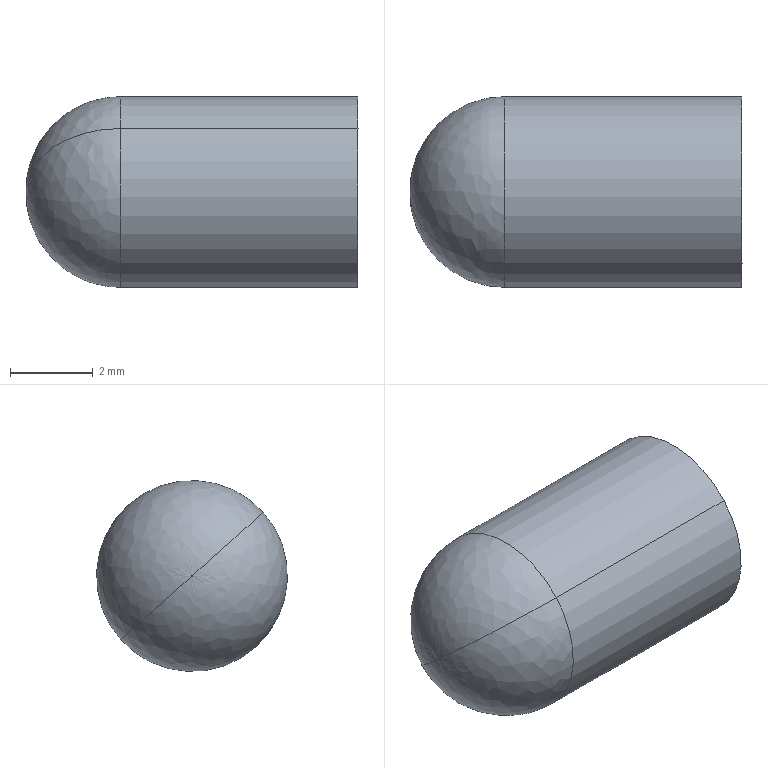Part | NX | features solid 2 | 1 solid | 11 faces | box 8 x 4.6 x 4.6 mm | volume 85.487 mm3 | cylinder 4 | plane 3 | spline 2 | cone 2 | commonest cylinder face diameters 2.6 x2 4.6 x2
STEP:
#1=CARTESIAN_POINT('',(270.755,52.052,28.635));
#2=VERTEX_POINT('',#1);
#3=CARTESIAN_POINT('',(276.475,52.052,28.635));
#4=VERTEX_POINT('',#3);
#5=CARTESIAN_POINT('',(276.475,52.052,28.635));
#6=DIRECTION('',(-1.,0.,0.));
#7=VECTOR('',#6,1000.);
#8=LINE('',#5,#7);
#9=EDGE_CURVE('',#2,#4,#8,.F.);
#10=ORIENTED_EDGE('',*,*,#9,.T.);
#11=CARTESIAN_POINT('',(276.475,55.486,25.575));
#12=VERTEX_POINT('',#11);
#13=CARTESIAN_POINT('',(276.475,53.769,27.105));
#14=DIRECTION('',(1.,0.,0.));
#15=DIRECTION('',(0.,0.7465,-0.6654));
#16=AXIS2_PLACEMENT_3D('',#13,#14,#15);
#17=CIRCLE('',#16,2.3);
#18=EDGE_CURVE('',#12,#4,#17,.T.);
#19=ORIENTED_EDGE('',*,*,#18,.F.);
#20=CARTESIAN_POINT('',(270.755,55.486,25.575));
#21=VERTEX_POINT('',#20);
#22=CARTESIAN_POINT('',(276.475,55.486,25.575));
#23=DIRECTION('',(-1.,0.,0.));
#24=VECTOR('',#23,1000.);
#25=LINE('',#22,#24);
#26=EDGE_CURVE('',#12,#21,#25,.T.);
#27=ORIENTED_EDGE('',*,*,#26,.T.);
#28=CARTESIAN_POINT('',(270.755,53.769,27.105));
#29=DIRECTION('',(-1.,0.,0.));
#30=DIRECTION('',(0.,-0.7465,0.6654));
#31=AXIS2_PLACEMENT_3D('',#28,#29,#30);
#32=CIRCLE('',#31,2.3);
#33=EDGE_CURVE('',#2,#21,#32,.T.);
#34=ORIENTED_EDGE('',*,*,#33,.F.);
#35=EDGE_LOOP('',(#10,#19,#27,#34));
#36=FACE_BOUND('',#35,.T.);
#37=CARTESIAN_POINT('',(276.475,53.769,27.105));
#38=DIRECTION('',(-1.,0.,0.));
#39=DIRECTION('',(0.,0.7465,-0.6654));
#40=AXIS2_PLACEMENT_3D('',#37,#38,#39);
#41=CYLINDRICAL_SURFACE('',#40,2.3);
#42=ADVANCED_FACE('',(#36),#41,.T.);
#43=CARTESIAN_POINT('',(268.475,53.755,27.118));
#44=VERTEX_POINT('',#43);
#45=CARTESIAN_POINT('',(270.755,53.755,27.118));
#46=DIRECTION('',(0.,0.6654,0.7465));
#47=DIRECTION('',(-1.,0.,0.));
#48=AXIS2_PLACEMENT_3D('',#45,#46,#47);
#49=CIRCLE('',#48,2.28);
#50=EDGE_CURVE('',#2,#44,#49,.F.);
#51=ORIENTED_EDGE('',*,*,#50,.F.);
#52=ORIENTED_EDGE('',*,*,#33,.T.);
#53=CARTESIAN_POINT('',(268.475,53.784,27.092));
#54=VERTEX_POINT('',#53);
#55=CARTESIAN_POINT('',(270.755,53.784,27.092));
#56=DIRECTION('',(0.,-0.6654,-0.7465));
#57=DIRECTION('',(-1.,0.,0.));
#58=AXIS2_PLACEMENT_3D('',#55,#56,#57);
#59=CIRCLE('',#58,2.28);
#60=EDGE_CURVE('',#54,#21,#59,.T.);
#61=ORIENTED_EDGE('',*,*,#60,.F.);
#62=CARTESIAN_POINT('',(268.475,53.769,27.105));
#63=DIRECTION('',(-1.,0.,0.));
#64=DIRECTION('',(0.,-0.7465,0.6654));
#65=AXIS2_PLACEMENT_3D('',#62,#63,#64);
#66=CIRCLE('',#65,0.01975);
#67=EDGE_CURVE('',#44,#54,#66,.T.);
#68=ORIENTED_EDGE('',*,*,#67,.F.);
#69=EDGE_LOOP('',(#51,#52,#61,#68));
#70=FACE_BOUND('',#69,.T.);
#71=CARTESIAN_POINT('',(268.475,53.77,27.095));
#72=CARTESIAN_POINT('',(268.469,53.911,25.728));
#73=CARTESIAN_POINT('',(269.454,54.009,24.775));
#74=CARTESIAN_POINT('',(270.827,54.005,24.818));
#75=CARTESIAN_POINT('',(268.475,53.78,27.096));
#76=CARTESIAN_POINT('',(268.469,55.305,25.872));
#77=CARTESIAN_POINT('',(269.454,56.369,25.018));
#78=CARTESIAN_POINT('',(270.827,56.321,25.057));
#79=CARTESIAN_POINT('',(268.475,53.783,27.106));
#80=CARTESIAN_POINT('',(268.469,55.736,27.205));
#81=CARTESIAN_POINT('',(269.454,57.098,27.275));
#82=CARTESIAN_POINT('',(270.827,57.037,27.272));
#83=CARTESIAN_POINT('',(268.475,53.776,27.112));
#84=CARTESIAN_POINT('',(268.469,54.69,28.138));
#85=CARTESIAN_POINT('',(269.454,55.328,28.853));
#86=CARTESIAN_POINT('',(270.827,55.299,28.821));
#87=CARTESIAN_POINT('',(268.475,53.768,27.119));
#88=CARTESIAN_POINT('',(268.469,53.644,29.071));
#89=CARTESIAN_POINT('',(269.454,53.557,30.432));
#90=CARTESIAN_POINT('',(270.827,53.561,30.37));
#91=CARTESIAN_POINT('',(268.475,53.759,27.115));
#92=CARTESIAN_POINT('',(268.469,52.369,28.489));
#93=CARTESIAN_POINT('',(269.454,51.398,29.448));
#94=CARTESIAN_POINT('',(270.827,51.442,29.405));
#95=CARTESIAN_POINT('',(268.475,53.759,27.105));
#96=CARTESIAN_POINT('',(268.469,52.386,27.088));
#97=CARTESIAN_POINT('',(269.454,51.427,27.076));
#98=CARTESIAN_POINT('',(270.827,51.471,27.077));
#99=(BOUNDED_SURFACE()B_SPLINE_SURFACE(3,3,((#71,#72,#73,#74),(#75,#76,#77,#78),(#79,#80,#81,#82),(#83,#84,#85,#86),(#87,#88,#89,#90),(#91,#92,#93,#94),(#95,#96,#97,#98)),.UNSPECIFIED.,.F.,.F.,.F.)B_SPLINE_SURFACE_WITH_KNOTS((4,3,4),(4,4),(0.,0.5,1.),(0.,1.),.PIECEWISE_BEZIER_KNOTS.)GEOMETRIC_REPRESENTATION_ITEM()RATIONAL_B_SPLINE_SURFACE(((1.682,1.339,1.339,1.682),(1.013,0.8067,0.8067,1.013),(1.013,0.8067,0.8067,1.013),(1.682,1.339,1.339,1.682),(1.013,0.8067,0.8067,1.013),(1.013,0.8067,0.8067,1.013),(1.682,1.339,1.339,1.682)))REPRESENTATION_ITEM('')SURFACE());
#100=ADVANCED_FACE('',(#70),#99,.T.);
#101=CARTESIAN_POINT('',(268.475,53.769,27.105));
#102=DIRECTION('',(-1.,0.,0.));
#103=DIRECTION('',(0.,0.7465,-0.6654));
#104=AXIS2_PLACEMENT_3D('',#101,#102,#103);
#105=CIRCLE('',#104,0.01975);
#106=EDGE_CURVE('',#54,#44,#105,.T.);
#107=ORIENTED_EDGE('',*,*,#106,.T.);
#108=ORIENTED_EDGE('',*,*,#67,.T.);
#109=EDGE_LOOP('',(#107,#108));
#110=FACE_BOUND('',#109,.T.);
#111=CARTESIAN_POINT('',(268.475,53.782,27.12));
#112=DIRECTION('',(1.,0.,0.));
#113=DIRECTION('',(0.,-0.7465,0.6654));
#114=AXIS2_PLACEMENT_3D('',#111,#112,#113);
#115=PLANE('',#114);
#116=ADVANCED_FACE('',(#110),#115,.F.);
#117=ORIENTED_EDGE('',*,*,#60,.T.);
#118=CARTESIAN_POINT('',(270.755,53.769,27.105));
#119=DIRECTION('',(-1.,0.,0.));
#120=DIRECTION('',(0.,0.7465,-0.6654));
#121=AXIS2_PLACEMENT_3D('',#118,#119,#120);
#122=CIRCLE('',#121,2.3);
#123=EDGE_CURVE('',#21,#2,#122,.T.);
#124=ORIENTED_EDGE('',*,*,#123,.T.);
#125=ORIENTED_EDGE('',*,*,#50,.T.);
#126=ORIENTED_EDGE('',*,*,#106,.F.);
#127=EDGE_LOOP('',(#117,#124,#125,#126));
#128=FACE_BOUND('',#127,.T.);
#129=CARTESIAN_POINT('',(268.475,53.768,27.115));
#130=CARTESIAN_POINT('',(268.469,53.628,28.482));
#131=CARTESIAN_POINT('',(269.454,53.53,29.435));
#132=CARTESIAN_POINT('',(270.827,53.534,29.392));
#133=CARTESIAN_POINT('',(268.475,53.758,27.114));
#134=CARTESIAN_POINT('',(268.469,52.234,28.338));
#135=CARTESIAN_POINT('',(269.454,51.17,29.192));
#136=CARTESIAN_POINT('',(270.827,51.218,29.153));
#137=CARTESIAN_POINT('',(268.475,53.755,27.104));
#138=CARTESIAN_POINT('',(268.469,51.802,27.005));
#139=CARTESIAN_POINT('',(269.454,50.44,26.935));
#140=CARTESIAN_POINT('',(270.827,50.502,26.938));
#141=CARTESIAN_POINT('',(268.475,53.763,27.098));
#142=CARTESIAN_POINT('',(268.469,52.849,26.072));
#143=CARTESIAN_POINT('',(269.454,52.211,25.357));
#144=CARTESIAN_POINT('',(270.827,52.24,25.389));
#145=CARTESIAN_POINT('',(268.475,53.77,27.091));
#146=CARTESIAN_POINT('',(268.469,53.895,25.139));
#147=CARTESIAN_POINT('',(269.454,53.982,23.778));
#148=CARTESIAN_POINT('',(270.827,53.978,23.84));
#149=CARTESIAN_POINT('',(268.475,53.779,27.095));
#150=CARTESIAN_POINT('',(268.469,55.17,25.721));
#151=CARTESIAN_POINT('',(269.454,56.14,24.762));
#152=CARTESIAN_POINT('',(270.827,56.096,24.805));
#153=CARTESIAN_POINT('',(268.475,53.779,27.105));
#154=CARTESIAN_POINT('',(268.469,55.153,27.122));
#155=CARTESIAN_POINT('',(269.454,56.111,27.134));
#156=CARTESIAN_POINT('',(270.827,56.068,27.133));
#157=(BOUNDED_SURFACE()B_SPLINE_SURFACE(3,3,((#129,#130,#131,#132),(#133,#134,#135,#136),(#137,#138,#139,#140),(#141,#142,#143,#144),(#145,#146,#147,#148),(#149,#150,#151,#152),(#153,#154,#155,#156)),.UNSPECIFIED.,.F.,.F.,.F.)B_SPLINE_SURFACE_WITH_KNOTS((4,3,4),(4,4),(0.,0.5,1.),(0.,1.),.PIECEWISE_BEZIER_KNOTS.)GEOMETRIC_REPRESENTATION_ITEM()RATIONAL_B_SPLINE_SURFACE(((1.682,1.339,1.339,1.682),(1.013,0.8067,0.8067,1.013),(1.013,0.8067,0.8067,1.013),(1.682,1.339,1.339,1.682),(1.013,0.8067,0.8067,1.013),(1.013,0.8067,0.8067,1.013),(1.682,1.339,1.339,1.682)))REPRESENTATION_ITEM('')SURFACE());
#158=ADVANCED_FACE('',(#128),#157,.T.);
#159=ORIENTED_EDGE('',*,*,#26,.F.);
#160=CARTESIAN_POINT('',(276.475,53.769,27.105));
#161=DIRECTION('',(1.,0.,0.));
#162=DIRECTION('',(0.,-0.7465,0.6654));
#163=AXIS2_PLACEMENT_3D('',#160,#161,#162);
#164=CIRCLE('',#163,2.3);
#165=EDGE_CURVE('',#4,#12,#164,.T.);
#166=ORIENTED_EDGE('',*,*,#165,.F.);
#167=ORIENTED_EDGE('',*,*,#9,.F.);
#168=ORIENTED_EDGE('',*,*,#123,.F.);
#169=EDGE_LOOP('',(#159,#166,#167,#168));
#170=FACE_BOUND('',#169,.T.);
#171=CARTESIAN_POINT('',(276.475,53.769,27.105));
#172=DIRECTION('',(-1.,0.,0.));
#173=DIRECTION('',(0.,0.7465,-0.6654));
#174=AXIS2_PLACEMENT_3D('',#171,#172,#173);
#175=CYLINDRICAL_SURFACE('',#174,2.3);
#176=ADVANCED_FACE('',(#170),#175,.T.);
#177=ORIENTED_EDGE('',*,*,#18,.T.);
#178=ORIENTED_EDGE('',*,*,#165,.T.);
#179=EDGE_LOOP('',(#177,#178));
#180=FACE_BOUND('',#179,.T.);
#181=CARTESIAN_POINT('',(276.475,54.964,26.04));
#182=VERTEX_POINT('',#181);
#183=CARTESIAN_POINT('',(276.475,52.575,28.17));
#184=VERTEX_POINT('',#183);
#185=CARTESIAN_POINT('',(276.475,53.769,27.105));
#186=DIRECTION('',(-1.,0.,0.));
#187=DIRECTION('',(0.,0.7465,-0.6654));
#188=AXIS2_PLACEMENT_3D('',#185,#186,#187);
#189=CIRCLE('',#188,1.6);
#190=EDGE_CURVE('',#182,#184,#189,.T.);
#191=ORIENTED_EDGE('',*,*,#190,.T.);
#192=CARTESIAN_POINT('',(276.475,53.769,27.105));
#193=DIRECTION('',(-1.,0.,0.));
#194=DIRECTION('',(0.,-0.7465,0.6654));
#195=AXIS2_PLACEMENT_3D('',#192,#193,#194);
#196=CIRCLE('',#195,1.6);
#197=EDGE_CURVE('',#184,#182,#196,.T.);
#198=ORIENTED_EDGE('',*,*,#197,.T.);
#199=EDGE_LOOP('',(#191,#198));
#200=FACE_BOUND('',#199,.T.);
#201=CARTESIAN_POINT('',(276.475,54.634,28.075));
#202=DIRECTION('',(-1.,0.,0.));
#203=DIRECTION('',(0.,0.7465,-0.6654));
#204=AXIS2_PLACEMENT_3D('',#201,#202,#203);
#205=PLANE('',#204);
#206=ADVANCED_FACE('',(#180,#200),#205,.F.);
#207=CARTESIAN_POINT('',(276.175,54.74,26.24));
#208=VERTEX_POINT('',#207);
#209=CARTESIAN_POINT('',(276.175,54.74,26.24));
#210=DIRECTION('',(0.7071,0.5279,-0.4705));
#211=VECTOR('',#210,1000.);
#212=LINE('',#209,#211);
#213=EDGE_CURVE('',#182,#208,#212,.F.);
#214=ORIENTED_EDGE('',*,*,#213,.F.);
#215=ORIENTED_EDGE('',*,*,#197,.F.);
#216=CARTESIAN_POINT('',(276.175,52.799,27.97));
#217=VERTEX_POINT('',#216);
#218=CARTESIAN_POINT('',(276.175,52.799,27.97));
#219=DIRECTION('',(0.7071,-0.5279,0.4705));
#220=VECTOR('',#219,1000.);
#221=LINE('',#218,#220);
#222=EDGE_CURVE('',#217,#184,#221,.T.);
#223=ORIENTED_EDGE('',*,*,#222,.F.);
#224=CARTESIAN_POINT('',(276.175,53.769,27.105));
#225=DIRECTION('',(-1.,0.,0.));
#226=DIRECTION('',(0.,-0.7465,0.6654));
#227=AXIS2_PLACEMENT_3D('',#224,#225,#226);
#228=CIRCLE('',#227,1.3);
#229=EDGE_CURVE('',#217,#208,#228,.T.);
#230=ORIENTED_EDGE('',*,*,#229,.T.);
#231=EDGE_LOOP('',(#214,#215,#223,#230));
#232=FACE_BOUND('',#231,.T.);
#233=CARTESIAN_POINT('',(276.325,53.769,27.105));
#234=DIRECTION('',(1.,0.,0.));
#235=DIRECTION('',(0.,-0.7465,0.6654));
#236=AXIS2_PLACEMENT_3D('',#233,#234,#235);
#237=CONICAL_SURFACE('',#236,1.45,0.7854);
#238=ADVANCED_FACE('',(#232),#237,.F.);
#239=CARTESIAN_POINT('',(269.975,52.799,27.97));
#240=VERTEX_POINT('',#239);
#241=CARTESIAN_POINT('',(276.175,52.799,27.97));
#242=DIRECTION('',(-1.,0.,0.));
#243=VECTOR('',#242,1000.);
#244=LINE('',#241,#243);
#245=EDGE_CURVE('',#217,#240,#244,.T.);
#246=ORIENTED_EDGE('',*,*,#245,.T.);
#247=CARTESIAN_POINT('',(269.975,54.74,26.24));
#248=VERTEX_POINT('',#247);
#249=CARTESIAN_POINT('',(269.975,53.769,27.105));
#250=DIRECTION('',(1.,0.,0.));
#251=DIRECTION('',(0.,0.7465,-0.6654));
#252=AXIS2_PLACEMENT_3D('',#249,#250,#251);
#253=CIRCLE('',#252,1.3);
#254=EDGE_CURVE('',#248,#240,#253,.T.);
#255=ORIENTED_EDGE('',*,*,#254,.F.);
#256=CARTESIAN_POINT('',(276.175,54.74,26.24));
#257=DIRECTION('',(-1.,0.,0.));
#258=VECTOR('',#257,1000.);
#259=LINE('',#256,#258);
#260=EDGE_CURVE('',#248,#208,#259,.F.);
#261=ORIENTED_EDGE('',*,*,#260,.T.);
#262=ORIENTED_EDGE('',*,*,#229,.F.);
#263=EDGE_LOOP('',(#246,#255,#261,#262));
#264=FACE_BOUND('',#263,.T.);
#265=CARTESIAN_POINT('',(276.475,53.769,27.105));
#266=DIRECTION('',(-1.,0.,0.));
#267=DIRECTION('',(0.,0.7465,-0.6654));
#268=AXIS2_PLACEMENT_3D('',#265,#266,#267);
#269=CYLINDRICAL_SURFACE('',#268,1.3);
#270=ADVANCED_FACE('',(#264),#269,.F.);
#271=ORIENTED_EDGE('',*,*,#260,.F.);
#272=CARTESIAN_POINT('',(269.975,53.769,27.105));
#273=DIRECTION('',(1.,0.,0.));
#274=DIRECTION('',(0.,-0.7465,0.6654));
#275=AXIS2_PLACEMENT_3D('',#272,#273,#274);
#276=CIRCLE('',#275,1.3);
#277=EDGE_CURVE('',#240,#248,#276,.T.);
#278=ORIENTED_EDGE('',*,*,#277,.F.);
#279=ORIENTED_EDGE('',*,*,#245,.F.);
#280=CARTESIAN_POINT('',(276.175,53.769,27.105));
#281=DIRECTION('',(-1.,0.,0.));
#282=DIRECTION('',(0.,0.7465,-0.6654));
#283=AXIS2_PLACEMENT_3D('',#280,#281,#282);
#284=CIRCLE('',#283,1.3);
#285=EDGE_CURVE('',#208,#217,#284,.T.);
#286=ORIENTED_EDGE('',*,*,#285,.F.);
#287=EDGE_LOOP('',(#271,#278,#279,#286));
#288=FACE_BOUND('',#287,.T.);
#289=CARTESIAN_POINT('',(276.475,53.769,27.105));
#290=DIRECTION('',(-1.,0.,0.));
#291=DIRECTION('',(0.,0.7465,-0.6654));
#292=AXIS2_PLACEMENT_3D('',#289,#290,#291);
#293=CYLINDRICAL_SURFACE('',#292,1.3);
#294=ADVANCED_FACE('',(#288),#293,.F.);
#295=ORIENTED_EDGE('',*,*,#222,.T.);
#296=ORIENTED_EDGE('',*,*,#190,.F.);
#297=ORIENTED_EDGE('',*,*,#213,.T.);
#298=ORIENTED_EDGE('',*,*,#285,.T.);
#299=EDGE_LOOP('',(#295,#296,#297,#298));
#300=FACE_BOUND('',#299,.T.);
#301=CARTESIAN_POINT('',(276.325,53.769,27.105));
#302=DIRECTION('',(1.,0.,0.));
#303=DIRECTION('',(0.,-0.7465,0.6654));
#304=AXIS2_PLACEMENT_3D('',#301,#302,#303);
#305=CONICAL_SURFACE('',#304,1.45,0.7854);
#306=ADVANCED_FACE('',(#300),#305,.F.);
#307=ORIENTED_EDGE('',*,*,#254,.T.);
#308=ORIENTED_EDGE('',*,*,#277,.T.);
#309=EDGE_LOOP('',(#307,#308));
#310=FACE_BOUND('',#309,.T.);
#311=CARTESIAN_POINT('',(269.975,53.769,27.105));
#312=DIRECTION('',(-1.,0.,0.));
#313=DIRECTION('',(0.,0.7465,-0.6654));
#314=AXIS2_PLACEMENT_3D('',#311,#312,#313);
#315=PLANE('',#314);
#316=ADVANCED_FACE('',(#310),#315,.F.);
#317=CLOSED_SHELL('',(#42,#100,#116,#158,#176,#206,#238,#270,#294,#306,#316));
#318=MANIFOLD_SOLID_BREP('',#317);
#319=(LENGTH_UNIT()NAMED_UNIT(*)SI_UNIT(.MILLI.,.METRE.));
#320=UNCERTAINTY_MEASURE_WITH_UNIT(LENGTH_MEASURE(0.00001),#319,'','');
#321=(NAMED_UNIT(*)PLANE_ANGLE_UNIT()SI_UNIT($,.RADIAN.));
#322=(NAMED_UNIT(*)SI_UNIT($,.STERADIAN.)SOLID_ANGLE_UNIT());
#323=(GEOMETRIC_REPRESENTATION_CONTEXT(3)GLOBAL_UNCERTAINTY_ASSIGNED_CONTEXT((#320))GLOBAL_UNIT_ASSIGNED_CONTEXT((#319,#321,#322))REPRESENTATION_CONTEXT('',''));
#324=ADVANCED_BREP_SHAPE_REPRESENTATION('',(#318),#323);